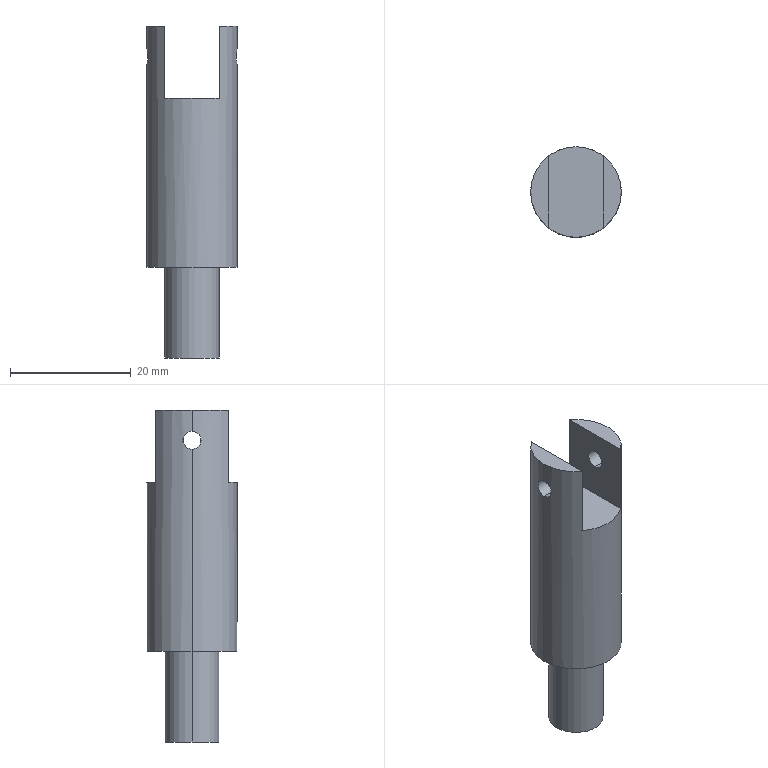Part | STEP file | Locking pin SGN-2-28 | 1 solid | 15 faces | box 15 x 15 x 55 mm | volume 6464 mm3 | cylinder 8 | plane 7 | commonest cylinder face diameters 3 x4 9 x2 15 x2